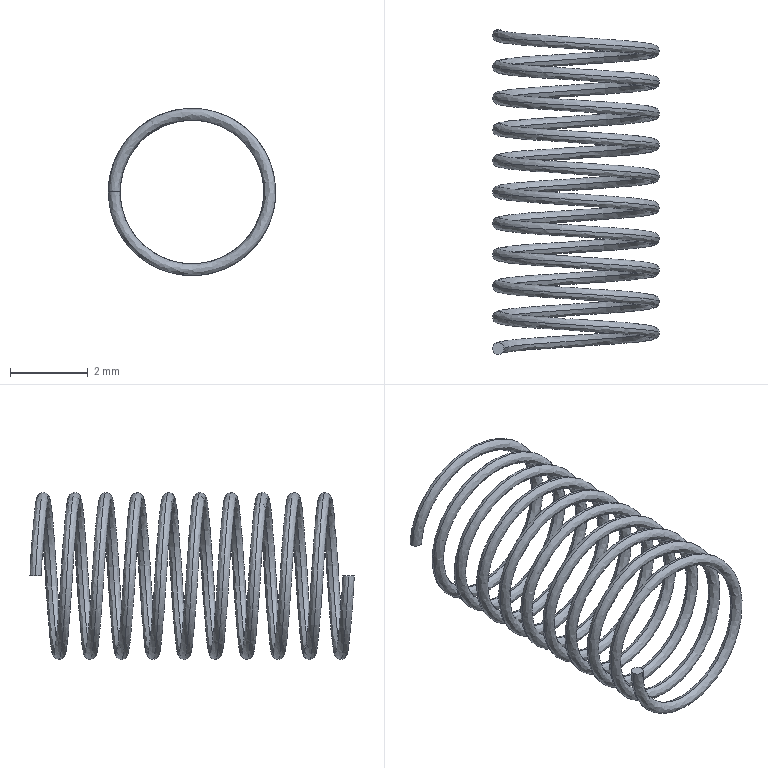Part | SolidWorks | features Sweep 1 | 1 solid | 4 faces | box 4.3 x 8.352 x 4.3 mm | volume 8.864 mm3 | spline 2 | plane 2